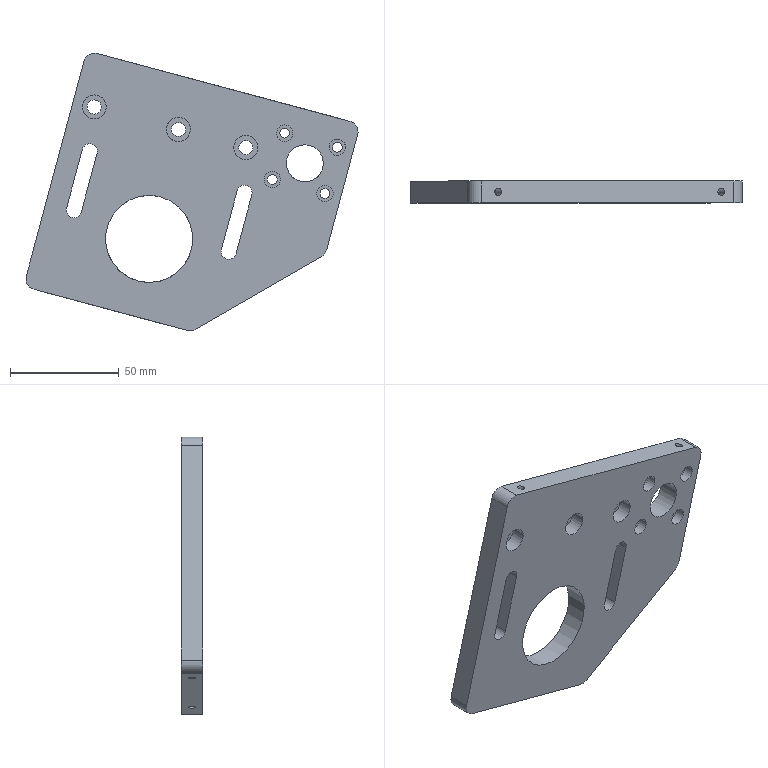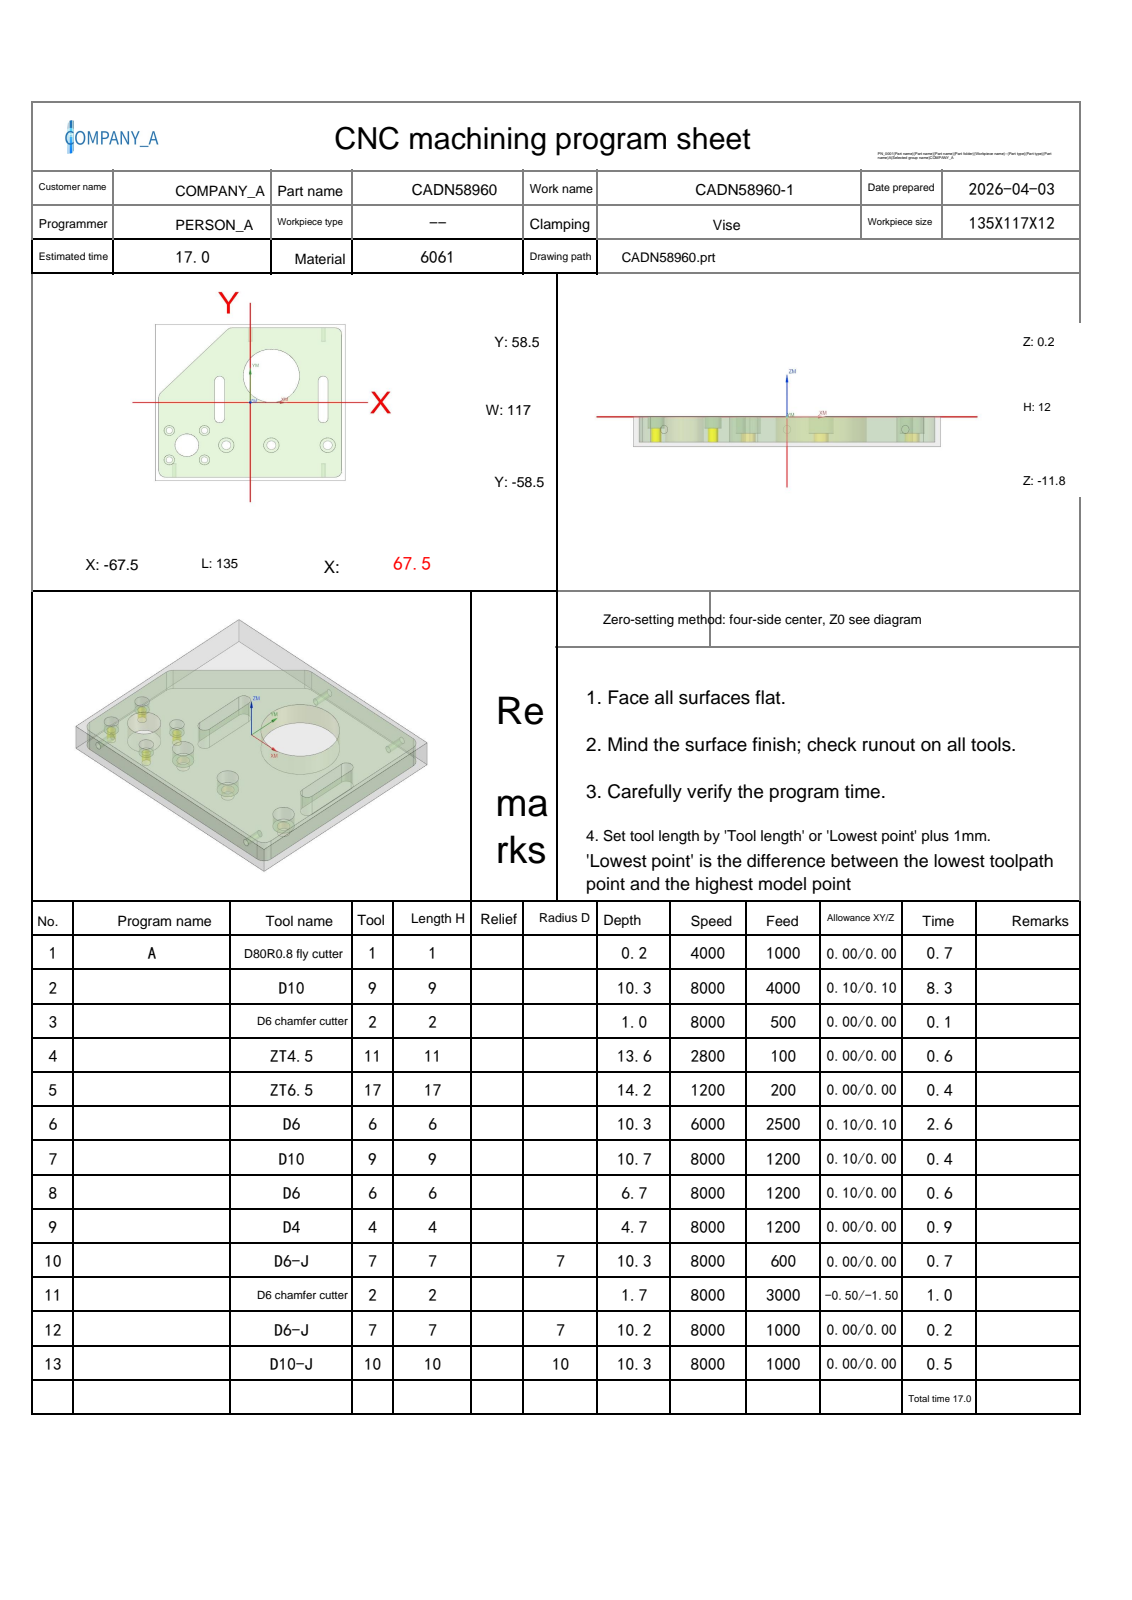NC program | NX | posted by the shop | part box 152.311 x 10 x 127.359 mm
Lines 1 to 39 of 4827:
%
O0001
(Machine time: 19.60 MIN)
(===Total Tool:9===)
(T1=D80R0.8 fly cutter D=80.  R=0.8  D-  H01 Z=-0.   )
(T9=D10     D=10.  R=0.   D-  H09 Z=-10.5 )
(T2=D6 chamfer cutter   D=6.   R=0.   D-  H02 Z=-1.5  )
(T11=ZT4.5  D=4.5  DR_a=118 D-  H11 Z=-13.35)
(T17=ZT6.5  D=6.5  DR_a=118 D-  H17 Z=-13.95)
(T6=D6      D=6.   R=0.   D-  H06 Z=-10.1 )
(T4=D4      D=4.   R=0.   D4  H04 Z=-4.5  )
(T7=D6-J    D=6.   R=0.   D7  H07 Z=-10.1 )
(T10=D10-J  D=10.  R=0.   D10 H10 Z=-10.1 )
G80 G90 G17 G49 G40
G91 G28 Z0
M01
N1 T01 M06
(D80R0.8 fly cutter  D=80. R=0.8 H=01 ce=0.00 di=0.00)
G00 G90 G54 X-110. Y48. M03 S4000
G43 H01 Z20.
M08
Z2.
G01 Z0.0 F1000.
X-105.
X105.
Y0.0
X-105.
Y-48.
X105.
X110.
Z2.
G00 Z20.
G91 G28 Z0.0
M05
M09
G91 G28 Z0.0
M01